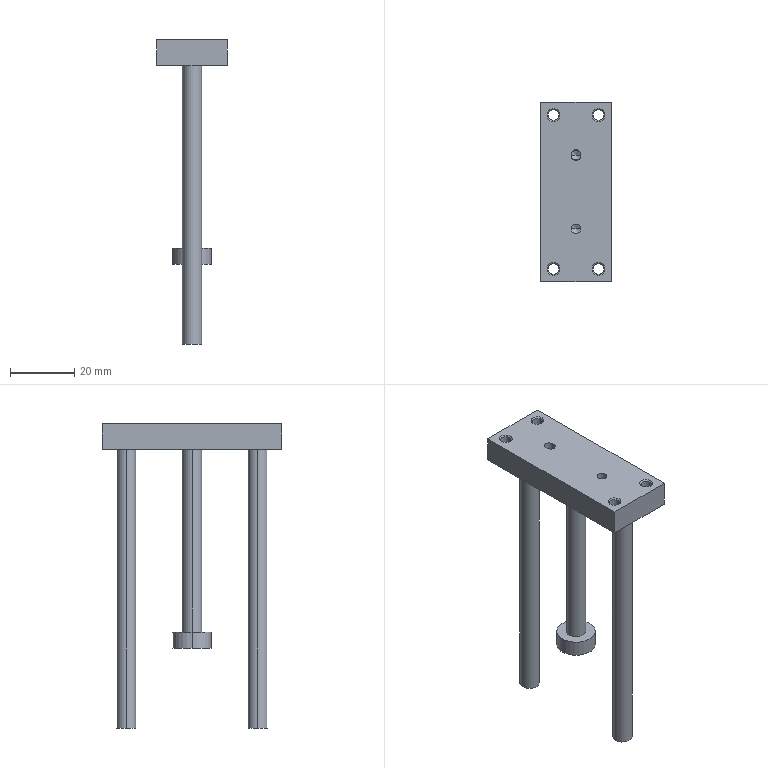Part | SolidWorks | features RevCut 6, ICE 5, RefAxis 3, 3DProfileFeature 1, Extrusion 1 | 1 solid | 56 faces | box 22 x 56 x 95 mm | volume 16589 mm3 | cylinder 22 | cone 20 | plane 14 | commonest cylinder face diameters 3.242 x8 3 x6 6 x6 12 x2
STEP:
#1=CARTESIAN_POINT('',(6.,0.,-65.));
#2=VERTEX_POINT('',#1);
#3=CARTESIAN_POINT('',(-6.,0.,-65.));
#4=VERTEX_POINT('',#3);
#5=CARTESIAN_POINT('',(0.,0.,-65.));
#6=DIRECTION('',(0.,0.,1.));
#7=DIRECTION('',(1.,0.,0.));
#8=AXIS2_PLACEMENT_3D('',#5,#6,#7);
#9=CIRCLE('',#8,6.);
#10=EDGE_CURVE('',#2,#4,#9,.T.);
#11=ORIENTED_EDGE('',*,*,#10,.F.);
#12=CARTESIAN_POINT('',(6.,0.,-70.));
#13=VERTEX_POINT('',#12);
#14=CARTESIAN_POINT('',(6.,0.,-65.));
#15=DIRECTION('',(0.,0.,-1.));
#16=VECTOR('',#15,1000.);
#17=LINE('',#14,#16);
#18=EDGE_CURVE('',#2,#13,#17,.T.);
#19=ORIENTED_EDGE('',*,*,#18,.T.);
#20=CARTESIAN_POINT('',(-6.,0.,-70.));
#21=VERTEX_POINT('',#20);
#22=CARTESIAN_POINT('',(0.,0.,-70.));
#23=DIRECTION('',(0.,0.,1.));
#24=DIRECTION('',(1.,0.,0.));
#25=AXIS2_PLACEMENT_3D('',#22,#23,#24);
#26=CIRCLE('',#25,6.);
#27=EDGE_CURVE('',#13,#21,#26,.T.);
#28=ORIENTED_EDGE('',*,*,#27,.T.);
#29=CARTESIAN_POINT('',(-6.,0.,-65.));
#30=DIRECTION('',(0.,0.,-1.));
#31=VECTOR('',#30,1000.);
#32=LINE('',#29,#31);
#33=EDGE_CURVE('',#4,#21,#32,.T.);
#34=ORIENTED_EDGE('',*,*,#33,.F.);
#35=EDGE_LOOP('',(#11,#19,#28,#34));
#36=FACE_OUTER_BOUND('',#35,.T.);
#37=CARTESIAN_POINT('',(0.,0.,-65.));
#38=DIRECTION('',(0.,0.,-1.));
#39=DIRECTION('',(-1.,0.,0.));
#40=AXIS2_PLACEMENT_3D('',#37,#38,#39);
#41=CYLINDRICAL_SURFACE('',#40,6.);
#42=ADVANCED_FACE('',(#36),#41,.T.);
#43=CARTESIAN_POINT('',(-3.,0.,-65.));
#44=VERTEX_POINT('',#43);
#45=CARTESIAN_POINT('',(3.,0.,-65.));
#46=VERTEX_POINT('',#45);
#47=CARTESIAN_POINT('',(0.,0.,-65.));
#48=DIRECTION('',(0.,0.,-1.));
#49=DIRECTION('',(1.,0.,0.));
#50=AXIS2_PLACEMENT_3D('',#47,#48,#49);
#51=CIRCLE('',#50,3.);
#52=EDGE_CURVE('',#44,#46,#51,.T.);
#53=ORIENTED_EDGE('',*,*,#52,.F.);
#54=CARTESIAN_POINT('',(-3.,0.,-8.));
#55=VERTEX_POINT('',#54);
#56=CARTESIAN_POINT('',(-3.,0.,-67.5));
#57=DIRECTION('',(0.,0.,1.));
#58=VECTOR('',#57,1000.);
#59=LINE('',#56,#58);
#60=EDGE_CURVE('',#44,#55,#59,.T.);
#61=ORIENTED_EDGE('',*,*,#60,.T.);
#62=CARTESIAN_POINT('',(3.,0.,-8.));
#63=VERTEX_POINT('',#62);
#64=CARTESIAN_POINT('',(0.,0.,-8.));
#65=DIRECTION('',(0.,0.,1.));
#66=DIRECTION('',(1.,0.,0.));
#67=AXIS2_PLACEMENT_3D('',#64,#65,#66);
#68=CIRCLE('',#67,3.);
#69=EDGE_CURVE('',#63,#55,#68,.T.);
#70=ORIENTED_EDGE('',*,*,#69,.F.);
#71=CARTESIAN_POINT('',(3.,0.,-67.5));
#72=DIRECTION('',(0.,0.,1.));
#73=VECTOR('',#72,1000.);
#74=LINE('',#71,#73);
#75=EDGE_CURVE('',#46,#63,#74,.T.);
#76=ORIENTED_EDGE('',*,*,#75,.F.);
#77=EDGE_LOOP('',(#53,#61,#70,#76));
#78=FACE_OUTER_BOUND('',#77,.T.);
#79=CARTESIAN_POINT('',(0.,0.,-67.5));
#80=DIRECTION('',(0.,0.,1.));
#81=DIRECTION('',(1.,0.,0.));
#82=AXIS2_PLACEMENT_3D('',#79,#80,#81);
#83=CYLINDRICAL_SURFACE('',#82,3.);
#84=ADVANCED_FACE('',(#78),#83,.T.);
#85=CARTESIAN_POINT('',(3.,-20.5,-95.));
#86=VERTEX_POINT('',#85);
#87=CARTESIAN_POINT('',(-3.,-20.5,-95.));
#88=VERTEX_POINT('',#87);
#89=CARTESIAN_POINT('',(0.,-20.5,-95.));
#90=DIRECTION('',(0.,0.,1.));
#91=DIRECTION('',(1.,0.,0.));
#92=AXIS2_PLACEMENT_3D('',#89,#90,#91);
#93=CIRCLE('',#92,3.);
#94=EDGE_CURVE('',#86,#88,#93,.T.);
#95=ORIENTED_EDGE('',*,*,#94,.T.);
#96=CARTESIAN_POINT('',(-3.,-20.5,-8.));
#97=VERTEX_POINT('',#96);
#98=CARTESIAN_POINT('',(-3.,-20.5,-95.));
#99=DIRECTION('',(0.,0.,1.));
#100=VECTOR('',#99,1000.);
#101=LINE('',#98,#100);
#102=EDGE_CURVE('',#88,#97,#101,.T.);
#103=ORIENTED_EDGE('',*,*,#102,.T.);
#104=CARTESIAN_POINT('',(3.,-20.5,-8.));
#105=VERTEX_POINT('',#104);
#106=CARTESIAN_POINT('',(0.,-20.5,-8.));
#107=DIRECTION('',(0.,0.,1.));
#108=DIRECTION('',(1.,0.,0.));
#109=AXIS2_PLACEMENT_3D('',#106,#107,#108);
#110=CIRCLE('',#109,3.);
#111=EDGE_CURVE('',#105,#97,#110,.T.);
#112=ORIENTED_EDGE('',*,*,#111,.F.);
#113=CARTESIAN_POINT('',(3.,-20.5,-95.));
#114=DIRECTION('',(0.,0.,1.));
#115=VECTOR('',#114,1000.);
#116=LINE('',#113,#115);
#117=EDGE_CURVE('',#86,#105,#116,.T.);
#118=ORIENTED_EDGE('',*,*,#117,.F.);
#119=EDGE_LOOP('',(#95,#103,#112,#118));
#120=FACE_OUTER_BOUND('',#119,.T.);
#121=CARTESIAN_POINT('',(0.,-20.5,-95.));
#122=DIRECTION('',(0.,0.,1.));
#123=DIRECTION('',(1.,0.,0.));
#124=AXIS2_PLACEMENT_3D('',#121,#122,#123);
#125=CYLINDRICAL_SURFACE('',#124,3.);
#126=ADVANCED_FACE('',(#120),#125,.T.);
#127=CARTESIAN_POINT('',(3.,20.5,-95.));
#128=VERTEX_POINT('',#127);
#129=CARTESIAN_POINT('',(-3.,20.5,-95.));
#130=VERTEX_POINT('',#129);
#131=CARTESIAN_POINT('',(0.,20.5,-95.));
#132=DIRECTION('',(0.,0.,1.));
#133=DIRECTION('',(1.,0.,0.));
#134=AXIS2_PLACEMENT_3D('',#131,#132,#133);
#135=CIRCLE('',#134,3.);
#136=EDGE_CURVE('',#128,#130,#135,.T.);
#137=ORIENTED_EDGE('',*,*,#136,.T.);
#138=CARTESIAN_POINT('',(-3.,20.5,-8.));
#139=VERTEX_POINT('',#138);
#140=CARTESIAN_POINT('',(-3.,20.5,-95.));
#141=DIRECTION('',(0.,0.,1.));
#142=VECTOR('',#141,1000.);
#143=LINE('',#140,#142);
#144=EDGE_CURVE('',#130,#139,#143,.T.);
#145=ORIENTED_EDGE('',*,*,#144,.T.);
#146=CARTESIAN_POINT('',(3.,20.5,-8.));
#147=VERTEX_POINT('',#146);
#148=CARTESIAN_POINT('',(0.,20.5,-8.));
#149=DIRECTION('',(0.,0.,1.));
#150=DIRECTION('',(1.,0.,0.));
#151=AXIS2_PLACEMENT_3D('',#148,#149,#150);
#152=CIRCLE('',#151,3.);
#153=EDGE_CURVE('',#147,#139,#152,.T.);
#154=ORIENTED_EDGE('',*,*,#153,.F.);
#155=CARTESIAN_POINT('',(3.,20.5,-95.));
#156=DIRECTION('',(0.,0.,1.));
#157=VECTOR('',#156,1000.);
#158=LINE('',#155,#157);
#159=EDGE_CURVE('',#128,#147,#158,.T.);
#160=ORIENTED_EDGE('',*,*,#159,.F.);
#161=EDGE_LOOP('',(#137,#145,#154,#160));
#162=FACE_OUTER_BOUND('',#161,.T.);
#163=CARTESIAN_POINT('',(0.,20.5,-95.));
#164=DIRECTION('',(0.,0.,1.));
#165=DIRECTION('',(1.,0.,0.));
#166=AXIS2_PLACEMENT_3D('',#163,#164,#165);
#167=CYLINDRICAL_SURFACE('',#166,3.);
#168=ADVANCED_FACE('',(#162),#167,.T.);
#169=CARTESIAN_POINT('',(-1.5,11.5,-6.));
#170=VERTEX_POINT('',#169);
#171=CARTESIAN_POINT('',(1.5,11.5,-6.));
#172=VERTEX_POINT('',#171);
#173=CARTESIAN_POINT('',(0.,11.5,-6.));
#174=DIRECTION('',(0.,0.,1.));
#175=DIRECTION('',(1.,0.,0.));
#176=AXIS2_PLACEMENT_3D('',#173,#174,#175);
#177=CIRCLE('',#176,1.5);
#178=EDGE_CURVE('',#170,#172,#177,.T.);
#179=ORIENTED_EDGE('',*,*,#178,.F.);
#180=CARTESIAN_POINT('',(-1.5,11.5,-3.));
#181=VERTEX_POINT('',#180);
#182=CARTESIAN_POINT('',(-1.5,11.5,-6.866));
#183=DIRECTION('',(0.,0.,1.));
#184=VECTOR('',#183,1000.);
#185=LINE('',#182,#184);
#186=EDGE_CURVE('',#170,#181,#185,.T.);
#187=ORIENTED_EDGE('',*,*,#186,.T.);
#188=CARTESIAN_POINT('',(1.5,11.5,-3.));
#189=VERTEX_POINT('',#188);
#190=CARTESIAN_POINT('',(0.,11.5,-3.));
#191=DIRECTION('',(0.,0.,1.));
#192=DIRECTION('',(1.,0.,0.));
#193=AXIS2_PLACEMENT_3D('',#190,#191,#192);
#194=CIRCLE('',#193,1.5);
#195=EDGE_CURVE('',#181,#189,#194,.T.);
#196=ORIENTED_EDGE('',*,*,#195,.T.);
#197=CARTESIAN_POINT('',(1.5,11.5,-6.866));
#198=DIRECTION('',(0.,0.,1.));
#199=VECTOR('',#198,1000.);
#200=LINE('',#197,#199);
#201=EDGE_CURVE('',#172,#189,#200,.T.);
#202=ORIENTED_EDGE('',*,*,#201,.F.);
#203=EDGE_LOOP('',(#179,#187,#196,#202));
#204=FACE_OUTER_BOUND('',#203,.T.);
#205=CARTESIAN_POINT('',(0.,11.5,-6.866));
#206=DIRECTION('',(0.,0.,1.));
#207=DIRECTION('',(1.,0.,0.));
#208=AXIS2_PLACEMENT_3D('',#205,#206,#207);
#209=CYLINDRICAL_SURFACE('',#208,1.5);
#210=ADVANCED_FACE('',(#204),#209,.F.);
#211=CARTESIAN_POINT('',(0.,11.5,-6.866));
#212=VERTEX_POINT('',#211);
#213=CARTESIAN_POINT('',(0.,11.5,-6.866));
#214=DIRECTION('',(0.866,0.,0.5));
#215=VECTOR('',#214,1000.);
#216=LINE('',#213,#215);
#217=EDGE_CURVE('',#212,#172,#216,.T.);
#218=ORIENTED_EDGE('',*,*,#217,.F.);
#219=CARTESIAN_POINT('',(0.,11.5,-6.866));
#220=DIRECTION('',(-0.866,0.,0.5));
#221=VECTOR('',#220,1000.);
#222=LINE('',#219,#221);
#223=EDGE_CURVE('',#212,#170,#222,.T.);
#224=ORIENTED_EDGE('',*,*,#223,.T.);
#225=ORIENTED_EDGE('',*,*,#178,.T.);
#226=EDGE_LOOP('',(#218,#224,#225));
#227=FACE_OUTER_BOUND('',#226,.T.);
#228=CARTESIAN_POINT('',(0.,11.5,993.134));
#229=DIRECTION('',(0.,0.,1.));
#230=DIRECTION('',(1.,0.,0.));
#231=AXIS2_PLACEMENT_3D('',#228,#229,#230);
#232=CONICAL_SURFACE('',#231,1732.051,1.047);
#233=ADVANCED_FACE('',(#227),#232,.F.);
#234=CARTESIAN_POINT('',(0.,-11.5,-6.866));
#235=VERTEX_POINT('',#234);
#236=CARTESIAN_POINT('',(1.5,-11.5,-6.));
#237=VERTEX_POINT('',#236);
#238=CARTESIAN_POINT('',(0.,-11.5,-6.866));
#239=DIRECTION('',(0.866,0.,0.5));
#240=VECTOR('',#239,1000.);
#241=LINE('',#238,#240);
#242=EDGE_CURVE('',#235,#237,#241,.T.);
#243=ORIENTED_EDGE('',*,*,#242,.F.);
#244=CARTESIAN_POINT('',(-1.5,-11.5,-6.));
#245=VERTEX_POINT('',#244);
#246=CARTESIAN_POINT('',(0.,-11.5,-6.866));
#247=DIRECTION('',(-0.866,0.,0.5));
#248=VECTOR('',#247,1000.);
#249=LINE('',#246,#248);
#250=EDGE_CURVE('',#235,#245,#249,.T.);
#251=ORIENTED_EDGE('',*,*,#250,.T.);
#252=CARTESIAN_POINT('',(0.,-11.5,-6.));
#253=DIRECTION('',(0.,0.,1.));
#254=DIRECTION('',(1.,0.,0.));
#255=AXIS2_PLACEMENT_3D('',#252,#253,#254);
#256=CIRCLE('',#255,1.5);
#257=EDGE_CURVE('',#245,#237,#256,.T.);
#258=ORIENTED_EDGE('',*,*,#257,.T.);
#259=EDGE_LOOP('',(#243,#251,#258));
#260=FACE_OUTER_BOUND('',#259,.T.);
#261=CARTESIAN_POINT('',(0.,-11.5,993.134));
#262=DIRECTION('',(0.,0.,1.));
#263=DIRECTION('',(1.,0.,0.));
#264=AXIS2_PLACEMENT_3D('',#261,#262,#263);
#265=CONICAL_SURFACE('',#264,1732.051,1.047);
#266=ADVANCED_FACE('',(#260),#265,.F.);
#267=ORIENTED_EDGE('',*,*,#257,.F.);
#268=CARTESIAN_POINT('',(-1.5,-11.5,0.));
#269=VERTEX_POINT('',#268);
#270=CARTESIAN_POINT('',(-1.5,-11.5,-6.866));
#271=DIRECTION('',(0.,0.,1.));
#272=VECTOR('',#271,1000.);
#273=LINE('',#270,#272);
#274=EDGE_CURVE('',#245,#269,#273,.T.);
#275=ORIENTED_EDGE('',*,*,#274,.T.);
#276=CARTESIAN_POINT('',(1.5,-11.5,0.));
#277=VERTEX_POINT('',#276);
#278=CARTESIAN_POINT('',(0.,-11.5,0.));
#279=DIRECTION('',(0.,0.,1.));
#280=DIRECTION('',(1.,0.,0.));
#281=AXIS2_PLACEMENT_3D('',#278,#279,#280);
#282=CIRCLE('',#281,1.5);
#283=EDGE_CURVE('',#269,#277,#282,.T.);
#284=ORIENTED_EDGE('',*,*,#283,.T.);
#285=CARTESIAN_POINT('',(1.5,-11.5,-6.866));
#286=DIRECTION('',(0.,0.,1.));
#287=VECTOR('',#286,1000.);
#288=LINE('',#285,#287);
#289=EDGE_CURVE('',#237,#277,#288,.T.);
#290=ORIENTED_EDGE('',*,*,#289,.F.);
#291=EDGE_LOOP('',(#267,#275,#284,#290));
#292=FACE_OUTER_BOUND('',#291,.T.);
#293=CARTESIAN_POINT('',(0.,-11.5,-6.866));
#294=DIRECTION('',(0.,0.,1.));
#295=DIRECTION('',(1.,0.,0.));
#296=AXIS2_PLACEMENT_3D('',#293,#294,#295);
#297=CYLINDRICAL_SURFACE('',#296,1.5);
#298=ADVANCED_FACE('',(#292),#297,.F.);
#299=CARTESIAN_POINT('',(5.379,24.,-7.621));
#300=VERTEX_POINT('',#299);
#301=CARTESIAN_POINT('',(8.621,24.,-7.621));
#302=VERTEX_POINT('',#301);
#303=CARTESIAN_POINT('',(7.,24.,-7.621));
#304=DIRECTION('',(0.,0.,1.));
#305=DIRECTION('',(1.,0.,0.));
#306=AXIS2_PLACEMENT_3D('',#303,#304,#305);
#307=CIRCLE('',#306,1.621);
#308=EDGE_CURVE('',#300,#302,#307,.T.);
#309=ORIENTED_EDGE('',*,*,#308,.T.);
#310=CARTESIAN_POINT('',(9.,24.,-8.));
#311=VERTEX_POINT('',#310);
#312=CARTESIAN_POINT('',(9.,24.,-8.));
#313=DIRECTION('',(0.7071,0.,-0.7071));
#314=VECTOR('',#313,1000.);
#315=LINE('',#312,#314);
#316=EDGE_CURVE('',#302,#311,#315,.T.);
#317=ORIENTED_EDGE('',*,*,#316,.T.);
#318=CARTESIAN_POINT('',(5.,24.,-8.));
#319=VERTEX_POINT('',#318);
#320=CARTESIAN_POINT('',(7.,24.,-8.));
#321=DIRECTION('',(0.,0.,1.));
#322=DIRECTION('',(1.,0.,0.));
#323=AXIS2_PLACEMENT_3D('',#320,#321,#322);
#324=CIRCLE('',#323,2.);
#325=EDGE_CURVE('',#319,#311,#324,.T.);
#326=ORIENTED_EDGE('',*,*,#325,.F.);
#327=CARTESIAN_POINT('',(5.,24.,-8.));
#328=DIRECTION('',(-0.7071,0.,-0.7071));
#329=VECTOR('',#328,1000.);
#330=LINE('',#327,#329);
#331=EDGE_CURVE('',#300,#319,#330,.T.);
#332=ORIENTED_EDGE('',*,*,#331,.F.);
#333=EDGE_LOOP('',(#309,#317,#326,#332));
#334=FACE_OUTER_BOUND('',#333,.T.);
#335=CARTESIAN_POINT('',(7.,24.,-8.));
#336=DIRECTION('',(0.,0.,-1.));
#337=DIRECTION('',(-1.,0.,0.));
#338=AXIS2_PLACEMENT_3D('',#335,#336,#337);
#339=CONICAL_SURFACE('',#338,2.,0.7854);
#340=ADVANCED_FACE('',(#334),#339,.F.);
#341=ORIENTED_EDGE('',*,*,#308,.F.);
#342=CARTESIAN_POINT('',(5.379,24.,-0.379));
#343=VERTEX_POINT('',#342);
#344=CARTESIAN_POINT('',(5.379,24.,-8.));
#345=DIRECTION('',(0.,0.,1.));
#346=VECTOR('',#345,1000.);
#347=LINE('',#344,#346);
#348=EDGE_CURVE('',#300,#343,#347,.T.);
#349=ORIENTED_EDGE('',*,*,#348,.T.);
#350=CARTESIAN_POINT('',(8.621,24.,-0.379));
#351=VERTEX_POINT('',#350);
#352=CARTESIAN_POINT('',(7.,24.,-0.379));
#353=DIRECTION('',(0.,0.,1.));
#354=DIRECTION('',(1.,0.,0.));
#355=AXIS2_PLACEMENT_3D('',#352,#353,#354);
#356=CIRCLE('',#355,1.621);
#357=EDGE_CURVE('',#343,#351,#356,.T.);
#358=ORIENTED_EDGE('',*,*,#357,.T.);
#359=CARTESIAN_POINT('',(8.621,24.,-8.));
#360=DIRECTION('',(0.,0.,1.));
#361=VECTOR('',#360,1000.);
#362=LINE('',#359,#361);
#363=EDGE_CURVE('',#302,#351,#362,.T.);
#364=ORIENTED_EDGE('',*,*,#363,.F.);
#365=EDGE_LOOP('',(#341,#349,#358,#364));
#366=FACE_OUTER_BOUND('',#365,.T.);
#367=CARTESIAN_POINT('',(7.,24.,-8.));
#368=DIRECTION('',(0.,0.,1.));
#369=DIRECTION('',(1.,0.,0.));
#370=AXIS2_PLACEMENT_3D('',#367,#368,#369);
#371=CYLINDRICAL_SURFACE('',#370,1.621);
#372=ADVANCED_FACE('',(#366),#371,.F.);
#373=ORIENTED_EDGE('',*,*,#357,.F.);
#374=CARTESIAN_POINT('',(5.,24.,0.));
#375=VERTEX_POINT('',#374);
#376=CARTESIAN_POINT('',(5.379,24.,-0.379));
#377=DIRECTION('',(-0.7071,0.,0.7071));
#378=VECTOR('',#377,1000.);
#379=LINE('',#376,#378);
#380=EDGE_CURVE('',#343,#375,#379,.T.);
#381=ORIENTED_EDGE('',*,*,#380,.T.);
#382=CARTESIAN_POINT('',(9.,24.,0.));
#383=VERTEX_POINT('',#382);
#384=CARTESIAN_POINT('',(7.,24.,0.));
#385=DIRECTION('',(0.,0.,1.));
#386=DIRECTION('',(1.,0.,0.));
#387=AXIS2_PLACEMENT_3D('',#384,#385,#386);
#388=CIRCLE('',#387,2.);
#389=EDGE_CURVE('',#375,#383,#388,.T.);
#390=ORIENTED_EDGE('',*,*,#389,.T.);
#391=CARTESIAN_POINT('',(8.621,24.,-0.379));
#392=DIRECTION('',(0.7071,0.,0.7071));
#393=VECTOR('',#392,1000.);
#394=LINE('',#391,#393);
#395=EDGE_CURVE('',#351,#383,#394,.T.);
#396=ORIENTED_EDGE('',*,*,#395,.F.);
#397=EDGE_LOOP('',(#373,#381,#390,#396));
#398=FACE_OUTER_BOUND('',#397,.T.);
#399=CARTESIAN_POINT('',(7.,24.,-0.379));
#400=DIRECTION('',(0.,0.,1.));
#401=DIRECTION('',(1.,0.,0.));
#402=AXIS2_PLACEMENT_3D('',#399,#400,#401);
#403=CONICAL_SURFACE('',#402,1.621,0.7854);
#404=ADVANCED_FACE('',(#398),#403,.F.);
#405=CARTESIAN_POINT('',(5.379,-24.,-7.621));
#406=VERTEX_POINT('',#405);
#407=CARTESIAN_POINT('',(8.621,-24.,-7.621));
#408=VERTEX_POINT('',#407);
#409=CARTESIAN_POINT('',(7.,-24.,-7.621));
#410=DIRECTION('',(0.,0.,1.));
#411=DIRECTION('',(1.,0.,0.));
#412=AXIS2_PLACEMENT_3D('',#409,#410,#411);
#413=CIRCLE('',#412,1.621);
#414=EDGE_CURVE('',#406,#408,#413,.T.);
#415=ORIENTED_EDGE('',*,*,#414,.T.);
#416=CARTESIAN_POINT('',(9.,-24.,-8.));
#417=VERTEX_POINT('',#416);
#418=CARTESIAN_POINT('',(9.,-24.,-8.));
#419=DIRECTION('',(0.7071,0.,-0.7071));
#420=VECTOR('',#419,1000.);
#421=LINE('',#418,#420);
#422=EDGE_CURVE('',#408,#417,#421,.T.);
#423=ORIENTED_EDGE('',*,*,#422,.T.);
#424=CARTESIAN_POINT('',(5.,-24.,-8.));
#425=VERTEX_POINT('',#424);
#426=CARTESIAN_POINT('',(7.,-24.,-8.));
#427=DIRECTION('',(0.,0.,1.));
#428=DIRECTION('',(1.,0.,0.));
#429=AXIS2_PLACEMENT_3D('',#426,#427,#428);
#430=CIRCLE('',#429,2.);
#431=EDGE_CURVE('',#425,#417,#430,.T.);
#432=ORIENTED_EDGE('',*,*,#431,.F.);
#433=CARTESIAN_POINT('',(5.,-24.,-8.));
#434=DIRECTION('',(-0.7071,0.,-0.7071));
#435=VECTOR('',#434,1000.);
#436=LINE('',#433,#435);
#437=EDGE_CURVE('',#406,#425,#436,.T.);
#438=ORIENTED_EDGE('',*,*,#437,.F.);
#439=EDGE_LOOP('',(#415,#423,#432,#438));
#440=FACE_OUTER_BOUND('',#439,.T.);
#441=CARTESIAN_POINT('',(7.,-24.,-8.));
#442=DIRECTION('',(0.,0.,-1.));
#443=DIRECTION('',(-1.,0.,0.));
#444=AXIS2_PLACEMENT_3D('',#441,#442,#443);
#445=CONICAL_SURFACE('',#444,2.,0.7854);
#446=ADVANCED_FACE('',(#440),#445,.F.);
#447=ORIENTED_EDGE('',*,*,#414,.F.);
#448=CARTESIAN_POINT('',(5.379,-24.,-0.379));
#449=VERTEX_POINT('',#448);
#450=CARTESIAN_POINT('',(5.379,-24.,-8.));
#451=DIRECTION('',(0.,0.,1.));
#452=VECTOR('',#451,1000.);
#453=LINE('',#450,#452);
#454=EDGE_CURVE('',#406,#449,#453,.T.);
#455=ORIENTED_EDGE('',*,*,#454,.T.);
#456=CARTESIAN_POINT('',(8.621,-24.,-0.379));
#457=VERTEX_POINT('',#456);
#458=CARTESIAN_POINT('',(7.,-24.,-0.379));
#459=DIRECTION('',(0.,0.,1.));
#460=DIRECTION('',(1.,0.,0.));
#461=AXIS2_PLACEMENT_3D('',#458,#459,#460);
#462=CIRCLE('',#461,1.621);
#463=EDGE_CURVE('',#449,#457,#462,.T.);
#464=ORIENTED_EDGE('',*,*,#463,.T.);
#465=CARTESIAN_POINT('',(8.621,-24.,-8.));
#466=DIRECTION('',(0.,0.,1.));
#467=VECTOR('',#466,1000.);
#468=LINE('',#465,#467);
#469=EDGE_CURVE('',#408,#457,#468,.T.);
#470=ORIENTED_EDGE('',*,*,#469,.F.);
#471=EDGE_LOOP('',(#447,#455,#464,#470));
#472=FACE_OUTER_BOUND('',#471,.T.);
#473=CARTESIAN_POINT('',(7.,-24.,-8.));
#474=DIRECTION('',(0.,0.,1.));
#475=DIRECTION('',(1.,0.,0.));
#476=AXIS2_PLACEMENT_3D('',#473,#474,#475);
#477=CYLINDRICAL_SURFACE('',#476,1.621);
#478=ADVANCED_FACE('',(#472),#477,.F.);
#479=ORIENTED_EDGE('',*,*,#463,.F.);
#480=CARTESIAN_POINT('',(5.,-24.,0.));
#481=VERTEX_POINT('',#480);
#482=CARTESIAN_POINT('',(5.379,-24.,-0.379));
#483=DIRECTION('',(-0.7071,0.,0.7071));
#484=VECTOR('',#483,1000.);
#485=LINE('',#482,#484);
#486=EDGE_CURVE('',#449,#481,#485,.T.);
#487=ORIENTED_EDGE('',*,*,#486,.T.);
#488=CARTESIAN_POINT('',(9.,-24.,0.));
#489=VERTEX_POINT('',#488);
#490=CARTESIAN_POINT('',(7.,-24.,0.));
#491=DIRECTION('',(0.,0.,1.));
#492=DIRECTION('',(1.,0.,0.));
#493=AXIS2_PLACEMENT_3D('',#490,#491,#492);
#494=CIRCLE('',#493,2.);
#495=EDGE_CURVE('',#481,#489,#494,.T.);
#496=ORIENTED_EDGE('',*,*,#495,.T.);
#497=CARTESIAN_POINT('',(8.621,-24.,-0.379));
#498=DIRECTION('',(0.7071,0.,0.7071));
#499=VECTOR('',#498,1000.);
#500=LINE('',#497,#499);
#501=EDGE_CURVE('',#457,#489,#500,.T.);
#502=ORIENTED_EDGE('',*,*,#501,.F.);
#503=EDGE_LOOP('',(#479,#487,#496,#502));
#504=FACE_OUTER_BOUND('',#503,.T.);
#505=CARTESIAN_POINT('',(7.,-24.,-0.379));
#506=DIRECTION('',(0.,0.,1.));
#507=DIRECTION('',(1.,0.,0.));
#508=AXIS2_PLACEMENT_3D('',#505,#506,#507);
#509=CONICAL_SURFACE('',#508,1.621,0.7854);
#510=ADVANCED_FACE('',(#504),#509,.F.);
#511=CARTESIAN_POINT('',(-8.621,-24.,-7.621));
#512=VERTEX_POINT('',#511);
#513=CARTESIAN_POINT('',(-5.379,-24.,-7.621));
#514=VERTEX_POINT('',#513);
#515=CARTESIAN_POINT('',(-7.,-24.,-7.621));
#516=DIRECTION('',(0.,0.,1.));
#517=DIRECTION('',(1.,0.,0.));
#518=AXIS2_PLACEMENT_3D('',#515,#516,#517);
#519=CIRCLE('',#518,1.621);
#520=EDGE_CURVE('',#512,#514,#519,.T.);
#521=ORIENTED_EDGE('',*,*,#520,.T.);
#522=CARTESIAN_POINT('',(-5.,-24.,-8.));
#523=VERTEX_POINT('',#522);
#524=CARTESIAN_POINT('',(-5.,-24.,-8.));
#525=DIRECTION('',(0.7071,0.,-0.7071));
#526=VECTOR('',#525,1000.);
#527=LINE('',#524,#526);
#528=EDGE_CURVE('',#514,#523,#527,.T.);
#529=ORIENTED_EDGE('',*,*,#528,.T.);
#530=CARTESIAN_POINT('',(-9.,-24.,-8.));
#531=VERTEX_POINT('',#530);
#532=CARTESIAN_POINT('',(-7.,-24.,-8.));
#533=DIRECTION('',(0.,0.,1.));
#534=DIRECTION('',(1.,0.,0.));
#535=AXIS2_PLACEMENT_3D('',#532,#533,#534);
#536=CIRCLE('',#535,2.);
#537=EDGE_CURVE('',#531,#523,#536,.T.);
#538=ORIENTED_EDGE('',*,*,#537,.F.);
#539=CARTESIAN_POINT('',(-9.,-24.,-8.));
#540=DIRECTION('',(-0.7071,0.,-0.7071));
#541=VECTOR('',#540,1000.);
#542=LINE('',#539,#541);
#543=EDGE_CURVE('',#512,#531,#542,.T.);
#544=ORIENTED_EDGE('',*,*,#543,.F.);
#545=EDGE_LOOP('',(#521,#529,#538,#544));
#546=FACE_OUTER_BOUND('',#545,.T.);
#547=CARTESIAN_POINT('',(-7.,-24.,-8.));
#548=DIRECTION('',(0.,0.,-1.));
#549=DIRECTION('',(-1.,0.,0.));
#550=AXIS2_PLACEMENT_3D('',#547,#548,#549);
#551=CONICAL_SURFACE('',#550,2.,0.7854);
#552=ADVANCED_FACE('',(#546),#551,.F.);
#553=ORIENTED_EDGE('',*,*,#520,.F.);
#554=CARTESIAN_POINT('',(-8.621,-24.,-0.379));
#555=VERTEX_POINT('',#554);
#556=CARTESIAN_POINT('',(-8.621,-24.,-8.));
#557=DIRECTION('',(0.,0.,1.));
#558=VECTOR('',#557,1000.);
#559=LINE('',#556,#558);
#560=EDGE_CURVE('',#512,#555,#559,.T.);
#561=ORIENTED_EDGE('',*,*,#560,.T.);
#562=CARTESIAN_POINT('',(-5.379,-24.,-0.379));
#563=VERTEX_POINT('',#562);
#564=CARTESIAN_POINT('',(-7.,-24.,-0.379));
#565=DIRECTION('',(0.,0.,1.));
#566=DIRECTION('',(1.,0.,0.));
#567=AXIS2_PLACEMENT_3D('',#564,#565,#566);
#568=CIRCLE('',#567,1.621);
#569=EDGE_CURVE('',#555,#563,#568,.T.);
#570=ORIENTED_EDGE('',*,*,#569,.T.);
#571=CARTESIAN_POINT('',(-5.379,-24.,-8.));
#572=DIRECTION('',(0.,0.,1.));
#573=VECTOR('',#572,1000.);
#574=LINE('',#571,#573);
#575=EDGE_CURVE('',#514,#563,#574,.T.);
#576=ORIENTED_EDGE('',*,*,#575,.F.);
#577=EDGE_LOOP('',(#553,#561,#570,#576));
#578=FACE_OUTER_BOUND('',#577,.T.);
#579=CARTESIAN_POINT('',(-7.,-24.,-8.));
#580=DIRECTION('',(0.,0.,1.));
#581=DIRECTION('',(1.,0.,0.));
#582=AXIS2_PLACEMENT_3D('',#579,#580,#581);
#583=CYLINDRICAL_SURFACE('',#582,1.621);
#584=ADVANCED_FACE('',(#578),#583,.F.);
#585=ORIENTED_EDGE('',*,*,#569,.F.);
#586=CARTESIAN_POINT('',(-9.,-24.,0.));
#587=VERTEX_POINT('',#586);
#588=CARTESIAN_POINT('',(-8.621,-24.,-0.379));
#589=DIRECTION('',(-0.7071,0.,0.7071));
#590=VECTOR('',#589,1000.);
#591=LINE('',#588,#590);
#592=EDGE_CURVE('',#555,#587,#591,.T.);
#593=ORIENTED_EDGE('',*,*,#592,.T.);
#594=CARTESIAN_POINT('',(-5.,-24.,0.));
#595=VERTEX_POINT('',#594);
#596=CARTESIAN_POINT('',(-7.,-24.,0.));
#597=DIRECTION('',(0.,0.,1.));
#598=DIRECTION('',(1.,0.,0.));
#599=AXIS2_PLACEMENT_3D('',#596,#597,#598);
#600=CIRCLE('',#599,2.);
#601=EDGE_CURVE('',#587,#595,#600,.T.);
#602=ORIENTED_EDGE('',*,*,#601,.T.);
#603=CARTESIAN_POINT('',(-5.379,-24.,-0.379));
#604=DIRECTION('',(0.7071,0.,0.7071));
#605=VECTOR('',#604,1000.);
#606=LINE('',#603,#605);
#607=EDGE_CURVE('',#563,#595,#606,.T.);
#608=ORIENTED_EDGE('',*,*,#607,.F.);
#609=EDGE_LOOP('',(#585,#593,#602,#608));
#610=FACE_OUTER_BOUND('',#609,.T.);
#611=CARTESIAN_POINT('',(-7.,-24.,-0.379));
#612=DIRECTION('',(0.,0.,1.));
#613=DIRECTION('',(1.,0.,0.));
#614=AXIS2_PLACEMENT_3D('',#611,#612,#613);
#615=CONICAL_SURFACE('',#614,1.621,0.7854);
#616=ADVANCED_FACE('',(#610),#615,.F.);
#617=CARTESIAN_POINT('',(-8.621,24.,-7.621));
#618=VERTEX_POINT('',#617);
#619=CARTESIAN_POINT('',(-5.379,24.,-7.621));
#620=VERTEX_POINT('',#619);
#621=CARTESIAN_POINT('',(-7.,24.,-7.621));
#622=DIRECTION('',(0.,0.,1.));
#623=DIRECTION('',(1.,0.,0.));
#624=AXIS2_PLACEMENT_3D('',#621,#622,#623);
#625=CIRCLE('',#624,1.621);
#626=EDGE_CURVE('',#618,#620,#625,.T.);
#627=ORIENTED_EDGE('',*,*,#626,.T.);
#628=CARTESIAN_POINT('',(-5.,24.,-8.));
#629=VERTEX_POINT('',#628);
#630=CARTESIAN_POINT('',(-5.,24.,-8.));
#631=DIRECTION('',(0.7071,0.,-0.7071));
#632=VECTOR('',#631,1000.);
#633=LINE('',#630,#632);
#634=EDGE_CURVE('',#620,#629,#633,.T.);
#635=ORIENTED_EDGE('',*,*,#634,.T.);
#636=CARTESIAN_POINT('',(-9.,24.,-8.));
#637=VERTEX_POINT('',#636);
#638=CARTESIAN_POINT('',(-7.,24.,-8.));
#639=DIRECTION('',(0.,0.,1.));
#640=DIRECTION('',(1.,0.,0.));
#641=AXIS2_PLACEMENT_3D('',#638,#639,#640);
#642=CIRCLE('',#641,2.);
#643=EDGE_CURVE('',#637,#629,#642,.T.);
#644=ORIENTED_EDGE('',*,*,#643,.F.);
#645=CARTESIAN_POINT('',(-9.,24.,-8.));
#646=DIRECTION('',(-0.7071,0.,-0.7071));
#647=VECTOR('',#646,1000.);
#648=LINE('',#645,#647);
#649=EDGE_CURVE('',#618,#637,#648,.T.);
#650=ORIENTED_EDGE('',*,*,#649,.F.);
#651=EDGE_LOOP('',(#627,#635,#644,#650));
#652=FACE_OUTER_BOUND('',#651,.T.);
#653=CARTESIAN_POINT('',(-7.,24.,-8.));
#654=DIRECTION('',(0.,0.,-1.));
#655=DIRECTION('',(-1.,0.,0.));
#656=AXIS2_PLACEMENT_3D('',#653,#654,#655);
#657=CONICAL_SURFACE('',#656,2.,0.7854);
#658=ADVANCED_FACE('',(#652),#657,.F.);
#659=ORIENTED_EDGE('',*,*,#626,.F.);
#660=CARTESIAN_POINT('',(-8.621,24.,-0.379));
#661=VERTEX_POINT('',#660);
#662=CARTESIAN_POINT('',(-8.621,24.,-8.));
#663=DIRECTION('',(0.,0.,1.));
#664=VECTOR('',#663,1000.);
#665=LINE('',#662,#664);
#666=EDGE_CURVE('',#618,#661,#665,.T.);
#667=ORIENTED_EDGE('',*,*,#666,.T.);
#668=CARTESIAN_POINT('',(-5.379,24.,-0.379));
#669=VERTEX_POINT('',#668);
#670=CARTESIAN_POINT('',(-7.,24.,-0.379));
#671=DIRECTION('',(0.,0.,1.));
#672=DIRECTION('',(1.,0.,0.));
#673=AXIS2_PLACEMENT_3D('',#670,#671,#672);
#674=CIRCLE('',#673,1.621);
#675=EDGE_CURVE('',#661,#669,#674,.T.);
#676=ORIENTED_EDGE('',*,*,#675,.T.);
#677=CARTESIAN_POINT('',(-5.379,24.,-8.));
#678=DIRECTION('',(0.,0.,1.));
#679=VECTOR('',#678,1000.);
#680=LINE('',#677,#679);
#681=EDGE_CURVE('',#620,#669,#680,.T.);
#682=ORIENTED_EDGE('',*,*,#681,.F.);
#683=EDGE_LOOP('',(#659,#667,#676,#682));
#684=FACE_OUTER_BOUND('',#683,.T.);
#685=CARTESIAN_POINT('',(-7.,24.,-8.));
#686=DIRECTION('',(0.,0.,1.));
#687=DIRECTION('',(1.,0.,0.));
#688=AXIS2_PLACEMENT_3D('',#685,#686,#687);
#689=CYLINDRICAL_SURFACE('',#688,1.621);
#690=ADVANCED_FACE('',(#684),#689,.F.);
#691=ORIENTED_EDGE('',*,*,#675,.F.);
#692=CARTESIAN_POINT('',(-9.,24.,0.));
#693=VERTEX_POINT('',#692);
#694=CARTESIAN_POINT('',(-8.621,24.,-0.379));
#695=DIRECTION('',(-0.7071,0.,0.7071));
#696=VECTOR('',#695,1000.);
#697=LINE('',#694,#696);
#698=EDGE_CURVE('',#661,#693,#697,.T.);
#699=ORIENTED_EDGE('',*,*,#698,.T.);
#700=CARTESIAN_POINT('',(-5.,24.,0.));
#701=VERTEX_POINT('',#700);
#702=CARTESIAN_POINT('',(-7.,24.,0.));
#703=DIRECTION('',(0.,0.,1.));
#704=DIRECTION('',(1.,0.,0.));
#705=AXIS2_PLACEMENT_3D('',#702,#703,#704);
#706=CIRCLE('',#705,2.);
#707=EDGE_CURVE('',#693,#701,#706,.T.);
#708=ORIENTED_EDGE('',*,*,#707,.T.);
#709=CARTESIAN_POINT('',(-5.379,24.,-0.379));
#710=DIRECTION('',(0.7071,0.,0.7071));
#711=VECTOR('',#710,1000.);
#712=LINE('',#709,#711);
#713=EDGE_CURVE('',#669,#701,#712,.T.);
#714=ORIENTED_EDGE('',*,*,#713,.F.);
#715=EDGE_LOOP('',(#691,#699,#708,#714));
#716=FACE_OUTER_BOUND('',#715,.T.);
#717=CARTESIAN_POINT('',(-7.,24.,-0.379));
#718=DIRECTION('',(0.,0.,1.));
#719=DIRECTION('',(1.,0.,0.));
#720=AXIS2_PLACEMENT_3D('',#717,#718,#719);
#721=CONICAL_SURFACE('',#720,1.621,0.7854);
#722=ADVANCED_FACE('',(#716),#721,.F.);
#723=CARTESIAN_POINT('',(-1.5,11.25,0.));
#724=VERTEX_POINT('',#723);
#725=CARTESIAN_POINT('',(1.5,11.25,0.));
#726=VERTEX_POINT('',#725);
#727=CARTESIAN_POINT('',(0.,11.25,0.));
#728=DIRECTION('',(0.,0.,1.));
#729=DIRECTION('',(1.,0.,0.));
#730=AXIS2_PLACEMENT_3D('',#727,#728,#729);
#731=CIRCLE('',#730,1.5);
#732=EDGE_CURVE('',#724,#726,#731,.T.);
#733=ORIENTED_EDGE('',*,*,#732,.F.);
#734=CARTESIAN_POINT('',(-1.5,11.75,0.));
#735=VERTEX_POINT('',#734);
#736=CARTESIAN_POINT('',(-1.5,11.75,0.));
#737=DIRECTION('',(0.,-1.,0.));
#738=VECTOR('',#737,1000.);
#739=LINE('',#736,#738);
#740=EDGE_CURVE('',#735,#724,#739,.T.);
#741=ORIENTED_EDGE('',*,*,#740,.F.);
#742=CARTESIAN_POINT('',(1.5,11.75,0.));
#743=VERTEX_POINT('',#742);
#744=CARTESIAN_POINT('',(0.,11.75,0.));
#745=DIRECTION('',(0.,0.,1.));
#746=DIRECTION('',(1.,0.,0.));
#747=AXIS2_PLACEMENT_3D('',#744,#745,#746);
#748=CIRCLE('',#747,1.5);
#749=EDGE_CURVE('',#743,#735,#748,.T.);
#750=ORIENTED_EDGE('',*,*,#749,.F.);
#751=CARTESIAN_POINT('',(1.5,11.25,0.));
#752=DIRECTION('',(0.,1.,0.));
#753=VECTOR('',#752,1000.);
#754=LINE('',#751,#753);
#755=EDGE_CURVE('',#726,#743,#754,.T.);
#756=ORIENTED_EDGE('',*,*,#755,.F.);
#757=EDGE_LOOP('',(#733,#741,#750,#756));
#758=FACE_BOUND('',#757,.T.);
#759=CARTESIAN_POINT('',(7.,-24.,0.));
#760=DIRECTION('',(0.,0.,1.));
#761=DIRECTION('',(1.,0.,0.));
#762=AXIS2_PLACEMENT_3D('',#759,#760,#761);
#763=CIRCLE('',#762,2.);
#764=EDGE_CURVE('',#489,#481,#763,.T.);
#765=ORIENTED_EDGE('',*,*,#764,.F.);
#766=ORIENTED_EDGE('',*,*,#495,.F.);
#767=EDGE_LOOP('',(#765,#766));
#768=FACE_BOUND('',#767,.T.);
#769=CARTESIAN_POINT('',(-7.,24.,0.));
#770=DIRECTION('',(0.,0.,1.));
#771=DIRECTION('',(1.,0.,0.));
#772=AXIS2_PLACEMENT_3D('',#769,#770,#771);
#773=CIRCLE('',#772,2.);
#774=EDGE_CURVE('',#701,#693,#773,.T.);
#775=ORIENTED_EDGE('',*,*,#774,.F.);
#776=ORIENTED_EDGE('',*,*,#707,.F.);
#777=EDGE_LOOP('',(#775,#776));
#778=FACE_BOUND('',#777,.T.);
#779=CARTESIAN_POINT('',(-11.,28.,0.));
#780=VERTEX_POINT('',#779);
#781=CARTESIAN_POINT('',(-11.,-28.,0.));
#782=VERTEX_POINT('',#781);
#783=CARTESIAN_POINT('',(-11.,28.,0.));
#784=DIRECTION('',(0.,-1.,0.));
#785=VECTOR('',#784,1000.);
#786=LINE('',#783,#785);
#787=EDGE_CURVE('',#780,#782,#786,.T.);
#788=ORIENTED_EDGE('',*,*,#787,.T.);
#789=CARTESIAN_POINT('',(11.,-28.,0.));
#790=VERTEX_POINT('',#789);
#791=CARTESIAN_POINT('',(-11.,-28.,0.));
#792=DIRECTION('',(1.,0.,0.));
#793=VECTOR('',#792,1000.);
#794=LINE('',#791,#793);
#795=EDGE_CURVE('',#782,#790,#794,.T.);
#796=ORIENTED_EDGE('',*,*,#795,.T.);
#797=CARTESIAN_POINT('',(11.,28.,0.));
#798=VERTEX_POINT('',#797);
#799=CARTESIAN_POINT('',(11.,-28.,0.));
#800=DIRECTION('',(0.,1.,0.));
#801=VECTOR('',#800,1000.);
#802=LINE('',#799,#801);
#803=EDGE_CURVE('',#790,#798,#802,.T.);
#804=ORIENTED_EDGE('',*,*,#803,.T.);
#805=CARTESIAN_POINT('',(11.,28.,0.));
#806=DIRECTION('',(-1.,0.,0.));
#807=VECTOR('',#806,1000.);
#808=LINE('',#805,#807);
#809=EDGE_CURVE('',#798,#780,#808,.T.);
#810=ORIENTED_EDGE('',*,*,#809,.T.);
#811=EDGE_LOOP('',(#788,#796,#804,#810));
#812=FACE_OUTER_BOUND('',#811,.T.);
#813=CARTESIAN_POINT('',(-7.,-24.,0.));
#814=DIRECTION('',(0.,0.,1.));
#815=DIRECTION('',(1.,0.,0.));
#816=AXIS2_PLACEMENT_3D('',#813,#814,#815);
#817=CIRCLE('',#816,2.);
#818=EDGE_CURVE('',#595,#587,#817,.T.);
#819=ORIENTED_EDGE('',*,*,#818,.F.);
#820=ORIENTED_EDGE('',*,*,#601,.F.);
#821=EDGE_LOOP('',(#819,#820));
#822=FACE_BOUND('',#821,.T.);
#823=CARTESIAN_POINT('',(7.,24.,0.));
#824=DIRECTION('',(0.,0.,1.));
#825=DIRECTION('',(1.,0.,0.));
#826=AXIS2_PLACEMENT_3D('',#823,#824,#825);
#827=CIRCLE('',#826,2.);
#828=EDGE_CURVE('',#383,#375,#827,.T.);
#829=ORIENTED_EDGE('',*,*,#828,.F.);
#830=ORIENTED_EDGE('',*,*,#389,.F.);
#831=EDGE_LOOP('',(#829,#830));
#832=FACE_BOUND('',#831,.T.);
#833=CARTESIAN_POINT('',(0.,-11.5,0.));
#834=DIRECTION('',(0.,0.,1.));
#835=DIRECTION('',(1.,0.,0.));
#836=AXIS2_PLACEMENT_3D('',#833,#834,#835);
#837=CIRCLE('',#836,1.5);
#838=EDGE_CURVE('',#277,#269,#837,.T.);
#839=ORIENTED_EDGE('',*,*,#838,.F.);
#840=ORIENTED_EDGE('',*,*,#283,.F.);
#841=EDGE_LOOP('',(#839,#840));
#842=FACE_BOUND('',#841,.T.);
#843=CARTESIAN_POINT('',(0.,0.,0.));
#844=DIRECTION('',(0.,0.,1.));
#845=DIRECTION('',(1.,0.,0.));
#846=AXIS2_PLACEMENT_3D('',#843,#844,#845);
#847=PLANE('',#846);
#848=ADVANCED_FACE('',(#758,#768,#778,#812,#822,#832,#842),#847,.T.);
#849=ORIENTED_EDGE('',*,*,#69,.T.);
#850=CARTESIAN_POINT('',(0.,0.,-8.));
#851=DIRECTION('',(0.,0.,1.));
#852=DIRECTION('',(1.,0.,0.));
#853=AXIS2_PLACEMENT_3D('',#850,#851,#852);
#854=CIRCLE('',#853,3.);
#855=EDGE_CURVE('',#55,#63,#854,.T.);
#856=ORIENTED_EDGE('',*,*,#855,.T.);
#857=EDGE_LOOP('',(#849,#856));
#858=FACE_BOUND('',#857,.T.);
#859=ORIENTED_EDGE('',*,*,#111,.T.);
#860=CARTESIAN_POINT('',(0.,-20.5,-8.));
#861=DIRECTION('',(0.,0.,1.));
#862=DIRECTION('',(1.,0.,0.));
#863=AXIS2_PLACEMENT_3D('',#860,#861,#862);
#864=CIRCLE('',#863,3.);
#865=EDGE_CURVE('',#97,#105,#864,.T.);
#866=ORIENTED_EDGE('',*,*,#865,.T.);
#867=EDGE_LOOP('',(#859,#866));
#868=FACE_BOUND('',#867,.T.);
#869=ORIENTED_EDGE('',*,*,#153,.T.);
#870=CARTESIAN_POINT('',(0.,20.5,-8.));
#871=DIRECTION('',(0.,0.,1.));
#872=DIRECTION('',(1.,0.,0.));
#873=AXIS2_PLACEMENT_3D('',#870,#871,#872);
#874=CIRCLE('',#873,3.);
#875=EDGE_CURVE('',#139,#147,#874,.T.);
#876=ORIENTED_EDGE('',*,*,#875,.T.);
#877=EDGE_LOOP('',(#869,#876));
#878=FACE_BOUND('',#877,.T.);
#879=ORIENTED_EDGE('',*,*,#431,.T.);
#880=CARTESIAN_POINT('',(7.,-24.,-8.));
#881=DIRECTION('',(0.,0.,1.));
#882=DIRECTION('',(1.,0.,0.));
#883=AXIS2_PLACEMENT_3D('',#880,#881,#882);
#884=CIRCLE('',#883,2.);
#885=EDGE_CURVE('',#417,#425,#884,.T.);
#886=ORIENTED_EDGE('',*,*,#885,.T.);
#887=EDGE_LOOP('',(#879,#886));
#888=FACE_BOUND('',#887,.T.);
#889=ORIENTED_EDGE('',*,*,#643,.T.);
#890=CARTESIAN_POINT('',(-7.,24.,-8.));
#891=DIRECTION('',(0.,0.,1.));
#892=DIRECTION('',(1.,0.,0.));
#893=AXIS2_PLACEMENT_3D('',#890,#891,#892);
#894=CIRCLE('',#893,2.);
#895=EDGE_CURVE('',#629,#637,#894,.T.);
#896=ORIENTED_EDGE('',*,*,#895,.T.);
#897=EDGE_LOOP('',(#889,#896));
#898=FACE_BOUND('',#897,.T.);
#899=CARTESIAN_POINT('',(-11.,28.,-8.));
#900=VERTEX_POINT('',#899);
#901=CARTESIAN_POINT('',(-11.,-28.,-8.));
#902=VERTEX_POINT('',#901);
#903=CARTESIAN_POINT('',(-11.,28.,-8.));
#904=DIRECTION('',(0.,-1.,0.));
#905=VECTOR('',#904,1000.);
#906=LINE('',#903,#905);
#907=EDGE_CURVE('',#900,#902,#906,.T.);
#908=ORIENTED_EDGE('',*,*,#907,.F.);
#909=CARTESIAN_POINT('',(11.,28.,-8.));
#910=VERTEX_POINT('',#909);
#911=CARTESIAN_POINT('',(11.,28.,-8.));
#912=DIRECTION('',(-1.,0.,0.));
#913=VECTOR('',#912,1000.);
#914=LINE('',#911,#913);
#915=EDGE_CURVE('',#910,#900,#914,.T.);
#916=ORIENTED_EDGE('',*,*,#915,.F.);
#917=CARTESIAN_POINT('',(11.,-28.,-8.));
#918=VERTEX_POINT('',#917);
#919=CARTESIAN_POINT('',(11.,-28.,-8.));
#920=DIRECTION('',(0.,1.,0.));
#921=VECTOR('',#920,1000.);
#922=LINE('',#919,#921);
#923=EDGE_CURVE('',#918,#910,#922,.T.);
#924=ORIENTED_EDGE('',*,*,#923,.F.);
#925=CARTESIAN_POINT('',(-11.,-28.,-8.));
#926=DIRECTION('',(1.,0.,0.));
#927=VECTOR('',#926,1000.);
#928=LINE('',#925,#927);
#929=EDGE_CURVE('',#902,#918,#928,.T.);
#930=ORIENTED_EDGE('',*,*,#929,.F.);
#931=EDGE_LOOP('',(#908,#916,#924,#930));
#932=FACE_OUTER_BOUND('',#931,.T.);
#933=ORIENTED_EDGE('',*,*,#537,.T.);
#934=CARTESIAN_POINT('',(-7.,-24.,-8.));
#935=DIRECTION('',(0.,0.,1.));
#936=DIRECTION('',(1.,0.,0.));
#937=AXIS2_PLACEMENT_3D('',#934,#935,#936);
#938=CIRCLE('',#937,2.);
#939=EDGE_CURVE('',#523,#531,#938,.T.);
#940=ORIENTED_EDGE('',*,*,#939,.T.);
#941=EDGE_LOOP('',(#933,#940));
#942=FACE_BOUND('',#941,.T.);
#943=ORIENTED_EDGE('',*,*,#325,.T.);
#944=CARTESIAN_POINT('',(7.,24.,-8.));
#945=DIRECTION('',(0.,0.,1.));
#946=DIRECTION('',(1.,0.,0.));
#947=AXIS2_PLACEMENT_3D('',#944,#945,#946);
#948=CIRCLE('',#947,2.);
#949=EDGE_CURVE('',#311,#319,#948,.T.);
#950=ORIENTED_EDGE('',*,*,#949,.T.);
#951=EDGE_LOOP('',(#943,#950));
#952=FACE_BOUND('',#951,.T.);
#953=CARTESIAN_POINT('',(0.,0.,-8.));
#954=DIRECTION('',(0.,0.,1.));
#955=DIRECTION('',(1.,0.,0.));
#956=AXIS2_PLACEMENT_3D('',#953,#954,#955);
#957=PLANE('',#956);
#958=ADVANCED_FACE('',(#858,#868,#878,#888,#898,#932,#942,#952),#957,.F.);
#959=ORIENTED_EDGE('',*,*,#787,.F.);
#960=CARTESIAN_POINT('',(-11.,28.,-8.));
#961=DIRECTION('',(0.,0.,1.));
#962=VECTOR('',#961,1000.);
#963=LINE('',#960,#962);
#964=EDGE_CURVE('',#900,#780,#963,.T.);
#965=ORIENTED_EDGE('',*,*,#964,.F.);
#966=ORIENTED_EDGE('',*,*,#907,.T.);
#967=CARTESIAN_POINT('',(-11.,-28.,-8.));
#968=DIRECTION('',(0.,0.,1.));
#969=VECTOR('',#968,1000.);
#970=LINE('',#967,#969);
#971=EDGE_CURVE('',#902,#782,#970,.T.);
#972=ORIENTED_EDGE('',*,*,#971,.T.);
#973=EDGE_LOOP('',(#959,#965,#966,#972));
#974=FACE_OUTER_BOUND('',#973,.T.);
#975=CARTESIAN_POINT('',(-11.,28.,-8.));
#976=DIRECTION('',(-1.,0.,0.));
#977=DIRECTION('',(0.,0.,1.));
#978=AXIS2_PLACEMENT_3D('',#975,#976,#977);
#979=PLANE('',#978);
#980=ADVANCED_FACE('',(#974),#979,.T.);
#981=ORIENTED_EDGE('',*,*,#809,.F.);
#982=CARTESIAN_POINT('',(11.,28.,-8.));
#983=DIRECTION('',(0.,0.,1.));
#984=VECTOR('',#983,1000.);
#985=LINE('',#982,#984);
#986=EDGE_CURVE('',#910,#798,#985,.T.);
#987=ORIENTED_EDGE('',*,*,#986,.F.);
#988=ORIENTED_EDGE('',*,*,#915,.T.);
#989=ORIENTED_EDGE('',*,*,#964,.T.);
#990=EDGE_LOOP('',(#981,#987,#988,#989));
#991=FACE_OUTER_BOUND('',#990,.T.);
#992=CARTESIAN_POINT('',(11.,28.,-8.));
#993=DIRECTION('',(0.,1.,0.));
#994=DIRECTION('',(0.,0.,1.));
#995=AXIS2_PLACEMENT_3D('',#992,#993,#994);
#996=PLANE('',#995);
#997=ADVANCED_FACE('',(#991),#996,.T.);
#998=ORIENTED_EDGE('',*,*,#803,.F.);
#999=CARTESIAN_POINT('',(11.,-28.,-8.));
#1000=DIRECTION('',(0.,0.,1.));
#1001=VECTOR('',#1000,1000.);
#1002=LINE('',#999,#1001);
#1003=EDGE_CURVE('',#918,#790,#1002,.T.);
#1004=ORIENTED_EDGE('',*,*,#1003,.F.);
#1005=ORIENTED_EDGE('',*,*,#923,.T.);
#1006=ORIENTED_EDGE('',*,*,#986,.T.);
#1007=EDGE_LOOP('',(#998,#1004,#1005,#1006));
#1008=FACE_OUTER_BOUND('',#1007,.T.);
#1009=CARTESIAN_POINT('',(11.,-28.,-8.));
#1010=DIRECTION('',(1.,0.,0.));
#1011=DIRECTION('',(0.,0.,-1.));
#1012=AXIS2_PLACEMENT_3D('',#1009,#1010,#1011);
#1013=PLANE('',#1012);
#1014=ADVANCED_FACE('',(#1008),#1013,.T.);
#1015=ORIENTED_EDGE('',*,*,#795,.F.);
#1016=ORIENTED_EDGE('',*,*,#971,.F.);
#1017=ORIENTED_EDGE('',*,*,#929,.T.);
#1018=ORIENTED_EDGE('',*,*,#1003,.T.);
#1019=EDGE_LOOP('',(#1015,#1016,#1017,#1018));
#1020=FACE_OUTER_BOUND('',#1019,.T.);
#1021=CARTESIAN_POINT('',(-11.,-28.,-8.));
#1022=DIRECTION('',(0.,-1.,0.));
#1023=DIRECTION('',(0.,0.,-1.));
#1024=AXIS2_PLACEMENT_3D('',#1021,#1022,#1023);
#1025=PLANE('',#1024);
#1026=ADVANCED_FACE('',(#1020),#1025,.T.);
#1027=ORIENTED_EDGE('',*,*,#698,.F.);
#1028=CARTESIAN_POINT('',(-7.,24.,-0.379));
#1029=DIRECTION('',(0.,0.,1.));
#1030=DIRECTION('',(1.,0.,0.));
#1031=AXIS2_PLACEMENT_3D('',#1028,#1029,#1030);
#1032=CIRCLE('',#1031,1.621);
#1033=EDGE_CURVE('',#669,#661,#1032,.T.);
#1034=ORIENTED_EDGE('',*,*,#1033,.F.);
#1035=ORIENTED_EDGE('',*,*,#713,.T.);
#1036=ORIENTED_EDGE('',*,*,#774,.T.);
#1037=EDGE_LOOP('',(#1027,#1034,#1035,#1036));
#1038=FACE_OUTER_BOUND('',#1037,.T.);
#1039=CARTESIAN_POINT('',(-7.,24.,-0.379));
#1040=DIRECTION('',(0.,0.,1.));
#1041=DIRECTION('',(1.,0.,0.));
#1042=AXIS2_PLACEMENT_3D('',#1039,#1040,#1041);
#1043=CONICAL_SURFACE('',#1042,1.621,0.7854);
#1044=ADVANCED_FACE('',(#1038),#1043,.F.);
#1045=ORIENTED_EDGE('',*,*,#666,.F.);
#1046=CARTESIAN_POINT('',(-7.,24.,-7.621));
#1047=DIRECTION('',(0.,0.,1.));
#1048=DIRECTION('',(1.,0.,0.));
#1049=AXIS2_PLACEMENT_3D('',#1046,#1047,#1048);
#1050=CIRCLE('',#1049,1.621);
#1051=EDGE_CURVE('',#620,#618,#1050,.T.);
#1052=ORIENTED_EDGE('',*,*,#1051,.F.);
#1053=ORIENTED_EDGE('',*,*,#681,.T.);
#1054=ORIENTED_EDGE('',*,*,#1033,.T.);
#1055=EDGE_LOOP('',(#1045,#1052,#1053,#1054));
#1056=FACE_OUTER_BOUND('',#1055,.T.);
#1057=CARTESIAN_POINT('',(-7.,24.,-8.));
#1058=DIRECTION('',(0.,0.,1.));
#1059=DIRECTION('',(1.,0.,0.));
#1060=AXIS2_PLACEMENT_3D('',#1057,#1058,#1059);
#1061=CYLINDRICAL_SURFACE('',#1060,1.621);
#1062=ADVANCED_FACE('',(#1056),#1061,.F.);
#1063=ORIENTED_EDGE('',*,*,#634,.F.);
#1064=ORIENTED_EDGE('',*,*,#1051,.T.);
#1065=ORIENTED_EDGE('',*,*,#649,.T.);
#1066=ORIENTED_EDGE('',*,*,#895,.F.);
#1067=EDGE_LOOP('',(#1063,#1064,#1065,#1066));
#1068=FACE_OUTER_BOUND('',#1067,.T.);
#1069=CARTESIAN_POINT('',(-7.,24.,-8.));
#1070=DIRECTION('',(0.,0.,-1.));
#1071=DIRECTION('',(-1.,0.,0.));
#1072=AXIS2_PLACEMENT_3D('',#1069,#1070,#1071);
#1073=CONICAL_SURFACE('',#1072,2.,0.7854);
#1074=ADVANCED_FACE('',(#1068),#1073,.F.);
#1075=ORIENTED_EDGE('',*,*,#592,.F.);
#1076=CARTESIAN_POINT('',(-7.,-24.,-0.379));
#1077=DIRECTION('',(0.,0.,1.));
#1078=DIRECTION('',(1.,0.,0.));
#1079=AXIS2_PLACEMENT_3D('',#1076,#1077,#1078);
#1080=CIRCLE('',#1079,1.621);
#1081=EDGE_CURVE('',#563,#555,#1080,.T.);
#1082=ORIENTED_EDGE('',*,*,#1081,.F.);
#1083=ORIENTED_EDGE('',*,*,#607,.T.);
#1084=ORIENTED_EDGE('',*,*,#818,.T.);
#1085=EDGE_LOOP('',(#1075,#1082,#1083,#1084));
#1086=FACE_OUTER_BOUND('',#1085,.T.);
#1087=CARTESIAN_POINT('',(-7.,-24.,-0.379));
#1088=DIRECTION('',(0.,0.,1.));
#1089=DIRECTION('',(1.,0.,0.));
#1090=AXIS2_PLACEMENT_3D('',#1087,#1088,#1089);
#1091=CONICAL_SURFACE('',#1090,1.621,0.7854);
#1092=ADVANCED_FACE('',(#1086),#1091,.F.);
#1093=ORIENTED_EDGE('',*,*,#560,.F.);
#1094=CARTESIAN_POINT('',(-7.,-24.,-7.621));
#1095=DIRECTION('',(0.,0.,1.));
#1096=DIRECTION('',(1.,0.,0.));
#1097=AXIS2_PLACEMENT_3D('',#1094,#1095,#1096);
#1098=CIRCLE('',#1097,1.621);
#1099=EDGE_CURVE('',#514,#512,#1098,.T.);
#1100=ORIENTED_EDGE('',*,*,#1099,.F.);
#1101=ORIENTED_EDGE('',*,*,#575,.T.);
#1102=ORIENTED_EDGE('',*,*,#1081,.T.);
#1103=EDGE_LOOP('',(#1093,#1100,#1101,#1102));
#1104=FACE_OUTER_BOUND('',#1103,.T.);
#1105=CARTESIAN_POINT('',(-7.,-24.,-8.));
#1106=DIRECTION('',(0.,0.,1.));
#1107=DIRECTION('',(1.,0.,0.));
#1108=AXIS2_PLACEMENT_3D('',#1105,#1106,#1107);
#1109=CYLINDRICAL_SURFACE('',#1108,1.621);
#1110=ADVANCED_FACE('',(#1104),#1109,.F.);
#1111=ORIENTED_EDGE('',*,*,#528,.F.);
#1112=ORIENTED_EDGE('',*,*,#1099,.T.);
#1113=ORIENTED_EDGE('',*,*,#543,.T.);
#1114=ORIENTED_EDGE('',*,*,#939,.F.);
#1115=EDGE_LOOP('',(#1111,#1112,#1113,#1114));
#1116=FACE_OUTER_BOUND('',#1115,.T.);
#1117=CARTESIAN_POINT('',(-7.,-24.,-8.));
#1118=DIRECTION('',(0.,0.,-1.));
#1119=DIRECTION('',(-1.,0.,0.));
#1120=AXIS2_PLACEMENT_3D('',#1117,#1118,#1119);
#1121=CONICAL_SURFACE('',#1120,2.,0.7854);
#1122=ADVANCED_FACE('',(#1116),#1121,.F.);
#1123=ORIENTED_EDGE('',*,*,#486,.F.);
#1124=CARTESIAN_POINT('',(7.,-24.,-0.379));
#1125=DIRECTION('',(0.,0.,1.));
#1126=DIRECTION('',(1.,0.,0.));
#1127=AXIS2_PLACEMENT_3D('',#1124,#1125,#1126);
#1128=CIRCLE('',#1127,1.621);
#1129=EDGE_CURVE('',#457,#449,#1128,.T.);
#1130=ORIENTED_EDGE('',*,*,#1129,.F.);
#1131=ORIENTED_EDGE('',*,*,#501,.T.);
#1132=ORIENTED_EDGE('',*,*,#764,.T.);
#1133=EDGE_LOOP('',(#1123,#1130,#1131,#1132));
#1134=FACE_OUTER_BOUND('',#1133,.T.);
#1135=CARTESIAN_POINT('',(7.,-24.,-0.379));
#1136=DIRECTION('',(0.,0.,1.));
#1137=DIRECTION('',(1.,0.,0.));
#1138=AXIS2_PLACEMENT_3D('',#1135,#1136,#1137);
#1139=CONICAL_SURFACE('',#1138,1.621,0.7854);
#1140=ADVANCED_FACE('',(#1134),#1139,.F.);
#1141=ORIENTED_EDGE('',*,*,#454,.F.);
#1142=CARTESIAN_POINT('',(7.,-24.,-7.621));
#1143=DIRECTION('',(0.,0.,1.));
#1144=DIRECTION('',(1.,0.,0.));
#1145=AXIS2_PLACEMENT_3D('',#1142,#1143,#1144);
#1146=CIRCLE('',#1145,1.621);
#1147=EDGE_CURVE('',#408,#406,#1146,.T.);
#1148=ORIENTED_EDGE('',*,*,#1147,.F.);
#1149=ORIENTED_EDGE('',*,*,#469,.T.);
#1150=ORIENTED_EDGE('',*,*,#1129,.T.);
#1151=EDGE_LOOP('',(#1141,#1148,#1149,#1150));
#1152=FACE_OUTER_BOUND('',#1151,.T.);
#1153=CARTESIAN_POINT('',(7.,-24.,-8.));
#1154=DIRECTION('',(0.,0.,1.));
#1155=DIRECTION('',(1.,0.,0.));
#1156=AXIS2_PLACEMENT_3D('',#1153,#1154,#1155);
#1157=CYLINDRICAL_SURFACE('',#1156,1.621);
#1158=ADVANCED_FACE('',(#1152),#1157,.F.);
#1159=ORIENTED_EDGE('',*,*,#422,.F.);
#1160=ORIENTED_EDGE('',*,*,#1147,.T.);
#1161=ORIENTED_EDGE('',*,*,#437,.T.);
#1162=ORIENTED_EDGE('',*,*,#885,.F.);
#1163=EDGE_LOOP('',(#1159,#1160,#1161,#1162));
#1164=FACE_OUTER_BOUND('',#1163,.T.);
#1165=CARTESIAN_POINT('',(7.,-24.,-8.));
#1166=DIRECTION('',(0.,0.,-1.));
#1167=DIRECTION('',(-1.,0.,0.));
#1168=AXIS2_PLACEMENT_3D('',#1165,#1166,#1167);
#1169=CONICAL_SURFACE('',#1168,2.,0.7854);
#1170=ADVANCED_FACE('',(#1164),#1169,.F.);
#1171=ORIENTED_EDGE('',*,*,#380,.F.);
#1172=CARTESIAN_POINT('',(7.,24.,-0.379));
#1173=DIRECTION('',(0.,0.,1.));
#1174=DIRECTION('',(1.,0.,0.));
#1175=AXIS2_PLACEMENT_3D('',#1172,#1173,#1174);
#1176=CIRCLE('',#1175,1.621);
#1177=EDGE_CURVE('',#351,#343,#1176,.T.);
#1178=ORIENTED_EDGE('',*,*,#1177,.F.);
#1179=ORIENTED_EDGE('',*,*,#395,.T.);
#1180=ORIENTED_EDGE('',*,*,#828,.T.);
#1181=EDGE_LOOP('',(#1171,#1178,#1179,#1180));
#1182=FACE_OUTER_BOUND('',#1181,.T.);
#1183=CARTESIAN_POINT('',(7.,24.,-0.379));
#1184=DIRECTION('',(0.,0.,1.));
#1185=DIRECTION('',(1.,0.,0.));
#1186=AXIS2_PLACEMENT_3D('',#1183,#1184,#1185);
#1187=CONICAL_SURFACE('',#1186,1.621,0.7854);
#1188=ADVANCED_FACE('',(#1182),#1187,.F.);
#1189=ORIENTED_EDGE('',*,*,#348,.F.);
#1190=CARTESIAN_POINT('',(7.,24.,-7.621));
#1191=DIRECTION('',(0.,0.,1.));
#1192=DIRECTION('',(1.,0.,0.));
#1193=AXIS2_PLACEMENT_3D('',#1190,#1191,#1192);
#1194=CIRCLE('',#1193,1.621);
#1195=EDGE_CURVE('',#302,#300,#1194,.T.);
#1196=ORIENTED_EDGE('',*,*,#1195,.F.);
#1197=ORIENTED_EDGE('',*,*,#363,.T.);
#1198=ORIENTED_EDGE('',*,*,#1177,.T.);
#1199=EDGE_LOOP('',(#1189,#1196,#1197,#1198));
#1200=FACE_OUTER_BOUND('',#1199,.T.);
#1201=CARTESIAN_POINT('',(7.,24.,-8.));
#1202=DIRECTION('',(0.,0.,1.));
#1203=DIRECTION('',(1.,0.,0.));
#1204=AXIS2_PLACEMENT_3D('',#1201,#1202,#1203);
#1205=CYLINDRICAL_SURFACE('',#1204,1.621);
#1206=ADVANCED_FACE('',(#1200),#1205,.F.);
#1207=ORIENTED_EDGE('',*,*,#316,.F.);
#1208=ORIENTED_EDGE('',*,*,#1195,.T.);
#1209=ORIENTED_EDGE('',*,*,#331,.T.);
#1210=ORIENTED_EDGE('',*,*,#949,.F.);
#1211=EDGE_LOOP('',(#1207,#1208,#1209,#1210));
#1212=FACE_OUTER_BOUND('',#1211,.T.);
#1213=CARTESIAN_POINT('',(7.,24.,-8.));
#1214=DIRECTION('',(0.,0.,-1.));
#1215=DIRECTION('',(-1.,0.,0.));
#1216=AXIS2_PLACEMENT_3D('',#1213,#1214,#1215);
#1217=CONICAL_SURFACE('',#1216,2.,0.7854);
#1218=ADVANCED_FACE('',(#1212),#1217,.F.);
#1219=ORIENTED_EDGE('',*,*,#274,.F.);
#1220=CARTESIAN_POINT('',(0.,-11.5,-6.));
#1221=DIRECTION('',(0.,0.,1.));
#1222=DIRECTION('',(1.,0.,0.));
#1223=AXIS2_PLACEMENT_3D('',#1220,#1221,#1222);
#1224=CIRCLE('',#1223,1.5);
#1225=EDGE_CURVE('',#237,#245,#1224,.T.);
#1226=ORIENTED_EDGE('',*,*,#1225,.F.);
#1227=ORIENTED_EDGE('',*,*,#289,.T.);
#1228=ORIENTED_EDGE('',*,*,#838,.T.);
#1229=EDGE_LOOP('',(#1219,#1226,#1227,#1228));
#1230=FACE_OUTER_BOUND('',#1229,.T.);
#1231=CARTESIAN_POINT('',(0.,-11.5,-6.866));
#1232=DIRECTION('',(0.,0.,1.));
#1233=DIRECTION('',(1.,0.,0.));
#1234=AXIS2_PLACEMENT_3D('',#1231,#1232,#1233);
#1235=CYLINDRICAL_SURFACE('',#1234,1.5);
#1236=ADVANCED_FACE('',(#1230),#1235,.F.);
#1237=ORIENTED_EDGE('',*,*,#250,.F.);
#1238=ORIENTED_EDGE('',*,*,#242,.T.);
#1239=ORIENTED_EDGE('',*,*,#1225,.T.);
#1240=EDGE_LOOP('',(#1237,#1238,#1239));
#1241=FACE_OUTER_BOUND('',#1240,.T.);
#1242=CARTESIAN_POINT('',(0.,-11.5,993.134));
#1243=DIRECTION('',(0.,0.,1.));
#1244=DIRECTION('',(1.,0.,0.));
#1245=AXIS2_PLACEMENT_3D('',#1242,#1243,#1244);
#1246=CONICAL_SURFACE('',#1245,1732.051,1.047);
#1247=ADVANCED_FACE('',(#1241),#1246,.F.);
#1248=CARTESIAN_POINT('',(-1.5,11.75,-3.));
#1249=VERTEX_POINT('',#1248);
#1250=CARTESIAN_POINT('',(-1.5,11.75,-3.));
#1251=DIRECTION('',(0.,-1.,0.));
#1252=VECTOR('',#1251,1000.);
#1253=LINE('',#1250,#1252);
#1254=EDGE_CURVE('',#1249,#181,#1253,.T.);
#1255=ORIENTED_EDGE('',*,*,#1254,.F.);
#1256=CARTESIAN_POINT('',(-1.5,11.75,-3.));
#1257=DIRECTION('',(0.,0.,1.));
#1258=VECTOR('',#1257,1000.);
#1259=LINE('',#1256,#1258);
#1260=EDGE_CURVE('',#1249,#735,#1259,.T.);
#1261=ORIENTED_EDGE('',*,*,#1260,.T.);
#1262=ORIENTED_EDGE('',*,*,#740,.T.);
#1263=CARTESIAN_POINT('',(-1.5,11.25,-3.));
#1264=VERTEX_POINT('',#1263);
#1265=CARTESIAN_POINT('',(-1.5,11.25,-3.));
#1266=DIRECTION('',(0.,0.,1.));
#1267=VECTOR('',#1266,1000.);
#1268=LINE('',#1265,#1267);
#1269=EDGE_CURVE('',#1264,#724,#1268,.T.);
#1270=ORIENTED_EDGE('',*,*,#1269,.F.);
#1271=CARTESIAN_POINT('',(-1.5,11.75,-3.));
#1272=DIRECTION('',(0.,-1.,0.));
#1273=VECTOR('',#1272,1000.);
#1274=LINE('',#1271,#1273);
#1275=EDGE_CURVE('',#181,#1264,#1274,.T.);
#1276=ORIENTED_EDGE('',*,*,#1275,.F.);
#1277=EDGE_LOOP('',(#1255,#1261,#1262,#1270,#1276));
#1278=FACE_OUTER_BOUND('',#1277,.T.);
#1279=CARTESIAN_POINT('',(-1.5,11.75,-3.));
#1280=DIRECTION('',(-1.,0.,0.));
#1281=DIRECTION('',(0.,0.,1.));
#1282=AXIS2_PLACEMENT_3D('',#1279,#1280,#1281);
#1283=PLANE('',#1282);
#1284=ADVANCED_FACE('',(#1278),#1283,.F.);
#1285=CARTESIAN_POINT('',(1.5,11.25,-3.));
#1286=VERTEX_POINT('',#1285);
#1287=CARTESIAN_POINT('',(1.5,11.25,-3.));
#1288=DIRECTION('',(0.,1.,0.));
#1289=VECTOR('',#1288,1000.);
#1290=LINE('',#1287,#1289);
#1291=EDGE_CURVE('',#1286,#189,#1290,.T.);
#1292=ORIENTED_EDGE('',*,*,#1291,.F.);
#1293=CARTESIAN_POINT('',(1.5,11.25,-3.));
#1294=DIRECTION('',(0.,0.,1.));
#1295=VECTOR('',#1294,1000.);
#1296=LINE('',#1293,#1295);
#1297=EDGE_CURVE('',#1286,#726,#1296,.T.);
#1298=ORIENTED_EDGE('',*,*,#1297,.T.);
#1299=ORIENTED_EDGE('',*,*,#755,.T.);
#1300=CARTESIAN_POINT('',(1.5,11.75,-3.));
#1301=VERTEX_POINT('',#1300);
#1302=CARTESIAN_POINT('',(1.5,11.75,-3.));
#1303=DIRECTION('',(0.,0.,1.));
#1304=VECTOR('',#1303,1000.);
#1305=LINE('',#1302,#1304);
#1306=EDGE_CURVE('',#1301,#743,#1305,.T.);
#1307=ORIENTED_EDGE('',*,*,#1306,.F.);
#1308=CARTESIAN_POINT('',(1.5,11.25,-3.));
#1309=DIRECTION('',(0.,1.,0.));
#1310=VECTOR('',#1309,1000.);
#1311=LINE('',#1308,#1310);
#1312=EDGE_CURVE('',#189,#1301,#1311,.T.);
#1313=ORIENTED_EDGE('',*,*,#1312,.F.);
#1314=EDGE_LOOP('',(#1292,#1298,#1299,#1307,#1313));
#1315=FACE_OUTER_BOUND('',#1314,.T.);
#1316=CARTESIAN_POINT('',(1.5,11.25,-3.));
#1317=DIRECTION('',(1.,0.,0.));
#1318=DIRECTION('',(0.,0.,-1.));
#1319=AXIS2_PLACEMENT_3D('',#1316,#1317,#1318);
#1320=PLANE('',#1319);
#1321=ADVANCED_FACE('',(#1315),#1320,.F.);
#1322=ORIENTED_EDGE('',*,*,#1312,.T.);
#1323=CARTESIAN_POINT('',(0.,11.75,-3.));
#1324=DIRECTION('',(0.,0.,1.));
#1325=DIRECTION('',(1.,0.,0.));
#1326=AXIS2_PLACEMENT_3D('',#1323,#1324,#1325);
#1327=CIRCLE('',#1326,1.5);
#1328=EDGE_CURVE('',#1301,#1249,#1327,.T.);
#1329=ORIENTED_EDGE('',*,*,#1328,.T.);
#1330=ORIENTED_EDGE('',*,*,#1254,.T.);
#1331=CARTESIAN_POINT('',(0.,11.5,-3.));
#1332=DIRECTION('',(0.,0.,1.));
#1333=DIRECTION('',(1.,0.,0.));
#1334=AXIS2_PLACEMENT_3D('',#1331,#1332,#1333);
#1335=CIRCLE('',#1334,1.5);
#1336=EDGE_CURVE('',#189,#181,#1335,.T.);
#1337=ORIENTED_EDGE('',*,*,#1336,.F.);
#1338=EDGE_LOOP('',(#1322,#1329,#1330,#1337));
#1339=FACE_OUTER_BOUND('',#1338,.T.);
#1340=CARTESIAN_POINT('',(0.,11.25,-3.));
#1341=DIRECTION('',(0.,0.,1.));
#1342=DIRECTION('',(1.,0.,0.));
#1343=AXIS2_PLACEMENT_3D('',#1340,#1341,#1342);
#1344=PLANE('',#1343);
#1345=ADVANCED_FACE('',(#1339),#1344,.T.);
#1346=ORIENTED_EDGE('',*,*,#732,.T.);
#1347=ORIENTED_EDGE('',*,*,#1297,.F.);
#1348=CARTESIAN_POINT('',(0.,11.25,-3.));
#1349=DIRECTION('',(0.,0.,1.));
#1350=DIRECTION('',(1.,0.,0.));
#1351=AXIS2_PLACEMENT_3D('',#1348,#1349,#1350);
#1352=CIRCLE('',#1351,1.5);
#1353=EDGE_CURVE('',#1264,#1286,#1352,.T.);
#1354=ORIENTED_EDGE('',*,*,#1353,.F.);
#1355=ORIENTED_EDGE('',*,*,#1269,.T.);
#1356=EDGE_LOOP('',(#1346,#1347,#1354,#1355));
#1357=FACE_OUTER_BOUND('',#1356,.T.);
#1358=CARTESIAN_POINT('',(0.,11.25,-3.));
#1359=DIRECTION('',(0.,0.,1.));
#1360=DIRECTION('',(1.,0.,0.));
#1361=AXIS2_PLACEMENT_3D('',#1358,#1359,#1360);
#1362=CYLINDRICAL_SURFACE('',#1361,1.5);
#1363=ADVANCED_FACE('',(#1357),#1362,.F.);
#1364=ORIENTED_EDGE('',*,*,#749,.T.);
#1365=ORIENTED_EDGE('',*,*,#1260,.F.);
#1366=ORIENTED_EDGE('',*,*,#1328,.F.);
#1367=ORIENTED_EDGE('',*,*,#1306,.T.);
#1368=EDGE_LOOP('',(#1364,#1365,#1366,#1367));
#1369=FACE_OUTER_BOUND('',#1368,.T.);
#1370=CARTESIAN_POINT('',(0.,11.75,-3.));
#1371=DIRECTION('',(0.,0.,1.));
#1372=DIRECTION('',(1.,0.,0.));
#1373=AXIS2_PLACEMENT_3D('',#1370,#1371,#1372);
#1374=CYLINDRICAL_SURFACE('',#1373,1.5);
#1375=ADVANCED_FACE('',(#1369),#1374,.F.);
#1376=ORIENTED_EDGE('',*,*,#1275,.T.);
#1377=ORIENTED_EDGE('',*,*,#1353,.T.);
#1378=ORIENTED_EDGE('',*,*,#1291,.T.);
#1379=ORIENTED_EDGE('',*,*,#195,.F.);
#1380=EDGE_LOOP('',(#1376,#1377,#1378,#1379));
#1381=FACE_OUTER_BOUND('',#1380,.T.);
#1382=CARTESIAN_POINT('',(0.,11.25,-3.));
#1383=DIRECTION('',(0.,0.,1.));
#1384=DIRECTION('',(1.,0.,0.));
#1385=AXIS2_PLACEMENT_3D('',#1382,#1383,#1384);
#1386=PLANE('',#1385);
#1387=ADVANCED_FACE('',(#1381),#1386,.T.);
#1388=ORIENTED_EDGE('',*,*,#223,.F.);
#1389=ORIENTED_EDGE('',*,*,#217,.T.);
#1390=CARTESIAN_POINT('',(0.,11.5,-6.));
#1391=DIRECTION('',(0.,0.,1.));
#1392=DIRECTION('',(1.,0.,0.));
#1393=AXIS2_PLACEMENT_3D('',#1390,#1391,#1392);
#1394=CIRCLE('',#1393,1.5);
#1395=EDGE_CURVE('',#172,#170,#1394,.T.);
#1396=ORIENTED_EDGE('',*,*,#1395,.T.);
#1397=EDGE_LOOP('',(#1388,#1389,#1396));
#1398=FACE_OUTER_BOUND('',#1397,.T.);
#1399=CARTESIAN_POINT('',(0.,11.5,993.134));
#1400=DIRECTION('',(0.,0.,1.));
#1401=DIRECTION('',(1.,0.,0.));
#1402=AXIS2_PLACEMENT_3D('',#1399,#1400,#1401);
#1403=CONICAL_SURFACE('',#1402,1732.051,1.047);
#1404=ADVANCED_FACE('',(#1398),#1403,.F.);
#1405=ORIENTED_EDGE('',*,*,#186,.F.);
#1406=ORIENTED_EDGE('',*,*,#1395,.F.);
#1407=ORIENTED_EDGE('',*,*,#201,.T.);
#1408=ORIENTED_EDGE('',*,*,#1336,.T.);
#1409=EDGE_LOOP('',(#1405,#1406,#1407,#1408));
#1410=FACE_OUTER_BOUND('',#1409,.T.);
#1411=CARTESIAN_POINT('',(0.,11.5,-6.866));
#1412=DIRECTION('',(0.,0.,1.));
#1413=DIRECTION('',(1.,0.,0.));
#1414=AXIS2_PLACEMENT_3D('',#1411,#1412,#1413);
#1415=CYLINDRICAL_SURFACE('',#1414,1.5);
#1416=ADVANCED_FACE('',(#1410),#1415,.F.);
#1417=ORIENTED_EDGE('',*,*,#144,.F.);
#1418=CARTESIAN_POINT('',(0.,20.5,-95.));
#1419=DIRECTION('',(0.,0.,1.));
#1420=DIRECTION('',(1.,0.,0.));
#1421=AXIS2_PLACEMENT_3D('',#1418,#1419,#1420);
#1422=CIRCLE('',#1421,3.);
#1423=EDGE_CURVE('',#130,#128,#1422,.T.);
#1424=ORIENTED_EDGE('',*,*,#1423,.T.);
#1425=ORIENTED_EDGE('',*,*,#159,.T.);
#1426=ORIENTED_EDGE('',*,*,#875,.F.);
#1427=EDGE_LOOP('',(#1417,#1424,#1425,#1426));
#1428=FACE_OUTER_BOUND('',#1427,.T.);
#1429=CARTESIAN_POINT('',(0.,20.5,-95.));
#1430=DIRECTION('',(0.,0.,1.));
#1431=DIRECTION('',(1.,0.,0.));
#1432=AXIS2_PLACEMENT_3D('',#1429,#1430,#1431);
#1433=CYLINDRICAL_SURFACE('',#1432,3.);
#1434=ADVANCED_FACE('',(#1428),#1433,.T.);
#1435=ORIENTED_EDGE('',*,*,#136,.F.);
#1436=ORIENTED_EDGE('',*,*,#1423,.F.);
#1437=EDGE_LOOP('',(#1435,#1436));
#1438=FACE_OUTER_BOUND('',#1437,.T.);
#1439=CARTESIAN_POINT('',(0.,20.5,-95.));
#1440=DIRECTION('',(0.,0.,1.));
#1441=DIRECTION('',(1.,0.,0.));
#1442=AXIS2_PLACEMENT_3D('',#1439,#1440,#1441);
#1443=PLANE('',#1442);
#1444=ADVANCED_FACE('',(#1438),#1443,.F.);
#1445=ORIENTED_EDGE('',*,*,#102,.F.);
#1446=CARTESIAN_POINT('',(0.,-20.5,-95.));
#1447=DIRECTION('',(0.,0.,1.));
#1448=DIRECTION('',(1.,0.,0.));
#1449=AXIS2_PLACEMENT_3D('',#1446,#1447,#1448);
#1450=CIRCLE('',#1449,3.);
#1451=EDGE_CURVE('',#88,#86,#1450,.T.);
#1452=ORIENTED_EDGE('',*,*,#1451,.T.);
#1453=ORIENTED_EDGE('',*,*,#117,.T.);
#1454=ORIENTED_EDGE('',*,*,#865,.F.);
#1455=EDGE_LOOP('',(#1445,#1452,#1453,#1454));
#1456=FACE_OUTER_BOUND('',#1455,.T.);
#1457=CARTESIAN_POINT('',(0.,-20.5,-95.));
#1458=DIRECTION('',(0.,0.,1.));
#1459=DIRECTION('',(1.,0.,0.));
#1460=AXIS2_PLACEMENT_3D('',#1457,#1458,#1459);
#1461=CYLINDRICAL_SURFACE('',#1460,3.);
#1462=ADVANCED_FACE('',(#1456),#1461,.T.);
#1463=ORIENTED_EDGE('',*,*,#94,.F.);
#1464=ORIENTED_EDGE('',*,*,#1451,.F.);
#1465=EDGE_LOOP('',(#1463,#1464));
#1466=FACE_OUTER_BOUND('',#1465,.T.);
#1467=CARTESIAN_POINT('',(0.,-20.5,-95.));
#1468=DIRECTION('',(0.,0.,1.));
#1469=DIRECTION('',(1.,0.,0.));
#1470=AXIS2_PLACEMENT_3D('',#1467,#1468,#1469);
#1471=PLANE('',#1470);
#1472=ADVANCED_FACE('',(#1466),#1471,.F.);
#1473=ORIENTED_EDGE('',*,*,#60,.F.);
#1474=CARTESIAN_POINT('',(0.,0.,-65.));
#1475=DIRECTION('',(0.,0.,-1.));
#1476=DIRECTION('',(1.,0.,0.));
#1477=AXIS2_PLACEMENT_3D('',#1474,#1475,#1476);
#1478=CIRCLE('',#1477,3.);
#1479=EDGE_CURVE('',#46,#44,#1478,.T.);
#1480=ORIENTED_EDGE('',*,*,#1479,.F.);
#1481=ORIENTED_EDGE('',*,*,#75,.T.);
#1482=ORIENTED_EDGE('',*,*,#855,.F.);
#1483=EDGE_LOOP('',(#1473,#1480,#1481,#1482));
#1484=FACE_OUTER_BOUND('',#1483,.T.);
#1485=CARTESIAN_POINT('',(0.,0.,-67.5));
#1486=DIRECTION('',(0.,0.,1.));
#1487=DIRECTION('',(1.,0.,0.));
#1488=AXIS2_PLACEMENT_3D('',#1485,#1486,#1487);
#1489=CYLINDRICAL_SURFACE('',#1488,3.);
#1490=ADVANCED_FACE('',(#1484),#1489,.T.);
#1491=ORIENTED_EDGE('',*,*,#18,.F.);
#1492=CARTESIAN_POINT('',(0.,0.,-65.));
#1493=DIRECTION('',(0.,0.,1.));
#1494=DIRECTION('',(1.,0.,0.));
#1495=AXIS2_PLACEMENT_3D('',#1492,#1493,#1494);
#1496=CIRCLE('',#1495,6.);
#1497=EDGE_CURVE('',#4,#2,#1496,.T.);
#1498=ORIENTED_EDGE('',*,*,#1497,.F.);
#1499=ORIENTED_EDGE('',*,*,#33,.T.);
#1500=CARTESIAN_POINT('',(0.,0.,-70.));
#1501=DIRECTION('',(0.,0.,1.));
#1502=DIRECTION('',(1.,0.,0.));
#1503=AXIS2_PLACEMENT_3D('',#1500,#1501,#1502);
#1504=CIRCLE('',#1503,6.);
#1505=EDGE_CURVE('',#21,#13,#1504,.T.);
#1506=ORIENTED_EDGE('',*,*,#1505,.T.);
#1507=EDGE_LOOP('',(#1491,#1498,#1499,#1506));
#1508=FACE_OUTER_BOUND('',#1507,.T.);
#1509=CARTESIAN_POINT('',(0.,0.,-65.));
#1510=DIRECTION('',(0.,0.,-1.));
#1511=DIRECTION('',(-1.,0.,0.));
#1512=AXIS2_PLACEMENT_3D('',#1509,#1510,#1511);
#1513=CYLINDRICAL_SURFACE('',#1512,6.);
#1514=ADVANCED_FACE('',(#1508),#1513,.T.);
#1515=ORIENTED_EDGE('',*,*,#1479,.T.);
#1516=ORIENTED_EDGE('',*,*,#52,.T.);
#1517=EDGE_LOOP('',(#1515,#1516));
#1518=FACE_BOUND('',#1517,.T.);
#1519=ORIENTED_EDGE('',*,*,#1497,.T.);
#1520=ORIENTED_EDGE('',*,*,#10,.T.);
#1521=EDGE_LOOP('',(#1519,#1520));
#1522=FACE_OUTER_BOUND('',#1521,.T.);
#1523=CARTESIAN_POINT('',(0.,0.,-65.));
#1524=DIRECTION('',(0.,0.,1.));
#1525=DIRECTION('',(1.,0.,0.));
#1526=AXIS2_PLACEMENT_3D('',#1523,#1524,#1525);
#1527=PLANE('',#1526);
#1528=ADVANCED_FACE('',(#1518,#1522),#1527,.T.);
#1529=ORIENTED_EDGE('',*,*,#1505,.F.);
#1530=ORIENTED_EDGE('',*,*,#27,.F.);
#1531=EDGE_LOOP('',(#1529,#1530));
#1532=FACE_OUTER_BOUND('',#1531,.T.);
#1533=CARTESIAN_POINT('',(0.,0.,-70.));
#1534=DIRECTION('',(0.,0.,1.));
#1535=DIRECTION('',(1.,0.,0.));
#1536=AXIS2_PLACEMENT_3D('',#1533,#1534,#1535);
#1537=PLANE('',#1536);
#1538=ADVANCED_FACE('',(#1532),#1537,.F.);
#1539=CLOSED_SHELL('',(#42,#84,#126,#168,#210,#233,#266,#298,#340,#372,#404,#446,#478,#510,#552,#584,#616,#658,#690,#722,#848,#958,#980,#997,#1014,#1026,#1044,#1062,#1074,#1092,#1110,#1122,#1140,#1158,#1170,#1188,#1206,#1218,#1236,#1247,#1284,#1321,#1345,#1363,#1375,#1387,#1404,#1416,#1434,#1444,#1462,#1472,#1490,#1514,#1528,#1538));
#1540=MANIFOLD_SOLID_BREP('',#1539);
#1541=CARTESIAN_POINT('',(0.,0.,0.));
#1542=DIRECTION('',(0.,0.,1.));
#1543=DIRECTION('',(1.,0.,0.));
#1544=AXIS2_PLACEMENT_3D('',#1541,#1542,#1543);
#1545=(LENGTH_UNIT()NAMED_UNIT(*)SI_UNIT(.MILLI.,.METRE.));
#1546=UNCERTAINTY_MEASURE_WITH_UNIT(LENGTH_MEASURE(0.00001),#1545,'','');
#1547=(NAMED_UNIT(*)PLANE_ANGLE_UNIT()SI_UNIT($,.RADIAN.));
#1548=(NAMED_UNIT(*)SI_UNIT($,.STERADIAN.)SOLID_ANGLE_UNIT());
#1549=(GEOMETRIC_REPRESENTATION_CONTEXT(3)GLOBAL_UNCERTAINTY_ASSIGNED_CONTEXT((#1546))GLOBAL_UNIT_ASSIGNED_CONTEXT((#1545,#1547,#1548))REPRESENTATION_CONTEXT('',''));
#1550=ADVANCED_BREP_SHAPE_REPRESENTATION('',(#1540,#1544),#1549);